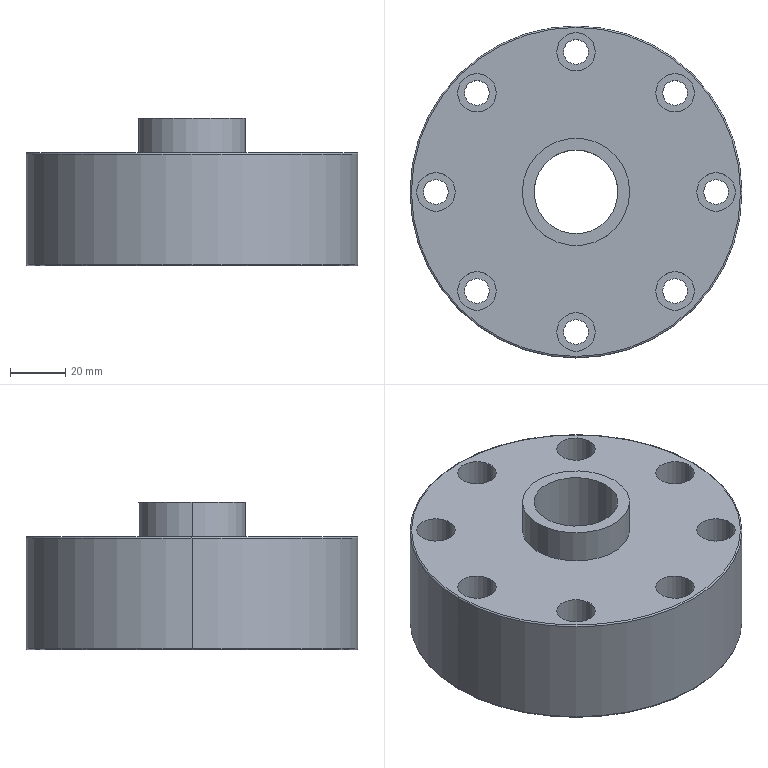Part | STEP file | 1 solid | 56 faces | box 120.6 x 120.6 x 53.5 mm | volume 414465 mm3 | cylinder 40 | plane 12 | torus 4 | commonest cylinder face diameters 9 x16 14 x16 30.5 x2 39 x2 50 x2 120.6 x2